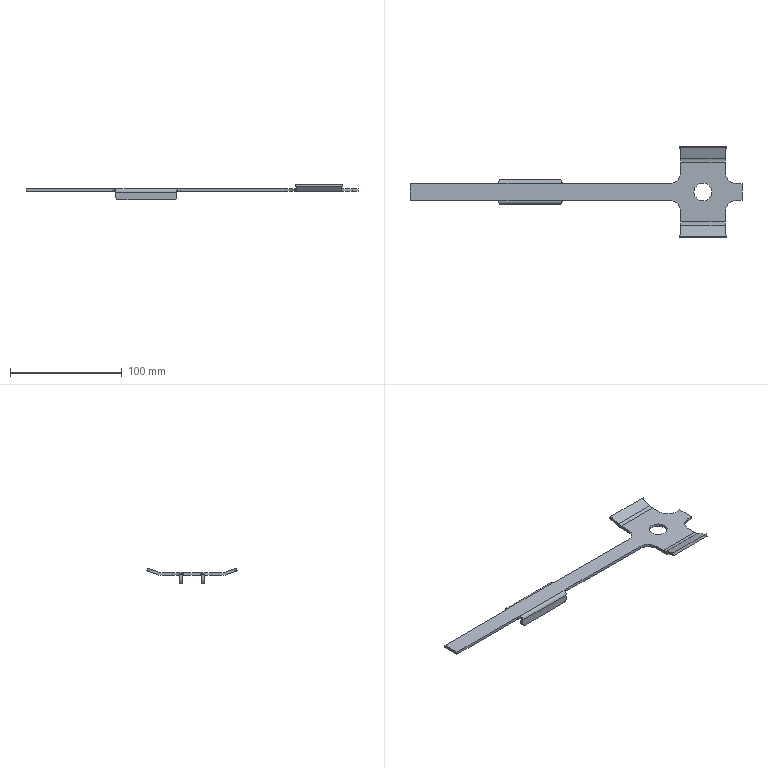Part | STEP file | lll_id946_x_t | 1 solid | 69 faces | box 297 x 81.263 x 14.104 mm | volume 20343 mm3 | plane 36 | cylinder 33 | commonest cylinder face diameters 6 x22 20 x6 1 x2 25 x2 16.1 x1